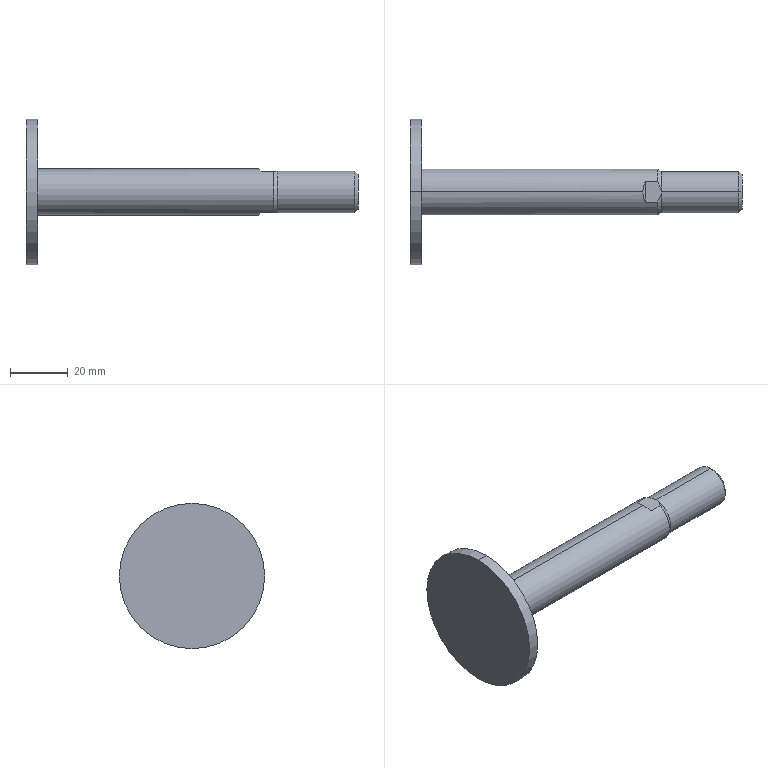Part | SolidWorks | features BaseBody 1 | 1 solid | 17 faces | box 115.2 x 50.4 x 50.4 mm | volume 29173 mm3 | plane 7 | cylinder 6 | cone 4 | commonest cylinder face diameters 14.4 x2 16 x2 50.4 x2
STEP:
#1=CARTESIAN_POINT('',(57.047,410.487,45.8));
#2=VERTEX_POINT('',#1);
#3=CARTESIAN_POINT('',(56.247,407.,45.));
#4=VERTEX_POINT('',#3);
#5=CARTESIAN_POINT('',(57.047,410.487,45.8));
#6=CARTESIAN_POINT('',(56.518,409.395,45.271));
#7=CARTESIAN_POINT('',(56.247,408.213,45.));
#8=CARTESIAN_POINT('',(56.247,407.,45.));
#9=(BOUNDED_CURVE()B_SPLINE_CURVE(3,(#5,#6,#7,#8),.UNSPECIFIED.,.F.,.F.)B_SPLINE_CURVE_WITH_KNOTS((4,4),(5.832,6.283),.UNSPECIFIED.)CURVE()GEOMETRIC_REPRESENTATION_ITEM()RATIONAL_B_SPLINE_CURVE((1.,0.9831,0.9831,1.))REPRESENTATION_ITEM(''));
#10=EDGE_CURVE('',#2,#4,#9,.T.);
#11=ORIENTED_EDGE('',*,*,#10,.T.);
#12=CARTESIAN_POINT('',(-20.553,407.,45.));
#13=VERTEX_POINT('',#12);
#14=CARTESIAN_POINT('',(-184.553,407.,45.));
#15=DIRECTION('',(-1.,0.,0.));
#16=VECTOR('',#15,1000.);
#17=LINE('',#14,#16);
#18=EDGE_CURVE('',#4,#13,#17,.T.);
#19=ORIENTED_EDGE('',*,*,#18,.T.);
#20=CARTESIAN_POINT('',(-20.553,407.,61.));
#21=VERTEX_POINT('',#20);
#22=CARTESIAN_POINT('',(-20.553,407.,53.));
#23=DIRECTION('',(1.,0.,0.));
#24=DIRECTION('',(0.,0.,1.));
#25=AXIS2_PLACEMENT_3D('',#22,#23,#24);
#26=CIRCLE('',#25,8.);
#27=EDGE_CURVE('',#13,#21,#26,.T.);
#28=ORIENTED_EDGE('',*,*,#27,.T.);
#29=CARTESIAN_POINT('',(56.247,407.,61.));
#30=VERTEX_POINT('',#29);
#31=CARTESIAN_POINT('',(-184.553,407.,61.));
#32=DIRECTION('',(-1.,0.,0.));
#33=VECTOR('',#32,1000.);
#34=LINE('',#31,#33);
#35=EDGE_CURVE('',#30,#21,#34,.T.);
#36=ORIENTED_EDGE('',*,*,#35,.F.);
#37=CARTESIAN_POINT('',(57.047,410.487,60.2));
#38=VERTEX_POINT('',#37);
#39=CARTESIAN_POINT('',(56.247,407.,61.));
#40=CARTESIAN_POINT('',(56.247,408.213,61.));
#41=CARTESIAN_POINT('',(56.518,409.395,60.729));
#42=CARTESIAN_POINT('',(57.047,410.487,60.2));
#43=(BOUNDED_CURVE()B_SPLINE_CURVE(3,(#39,#40,#41,#42),.UNSPECIFIED.,.F.,.F.)B_SPLINE_CURVE_WITH_KNOTS((4,4),(0.,0.451),.UNSPECIFIED.)CURVE()GEOMETRIC_REPRESENTATION_ITEM()RATIONAL_B_SPLINE_CURVE((1.,0.9831,0.9831,1.))REPRESENTATION_ITEM(''));
#44=EDGE_CURVE('',#30,#38,#43,.T.);
#45=ORIENTED_EDGE('',*,*,#44,.T.);
#46=CARTESIAN_POINT('',(61.261,410.487,60.2));
#47=VERTEX_POINT('',#46);
#48=CARTESIAN_POINT('',(-184.553,410.487,60.2));
#49=DIRECTION('',(1.,0.,0.));
#50=VECTOR('',#49,1000.);
#51=LINE('',#48,#50);
#52=EDGE_CURVE('',#38,#47,#51,.T.);
#53=ORIENTED_EDGE('',*,*,#52,.T.);
#54=CARTESIAN_POINT('',(61.261,410.487,45.8));
#55=VERTEX_POINT('',#54);
#56=CARTESIAN_POINT('',(61.261,407.,53.));
#57=DIRECTION('',(-1.,0.,0.));
#58=DIRECTION('',(0.,0.,1.));
#59=AXIS2_PLACEMENT_3D('',#56,#57,#58);
#60=CIRCLE('',#59,8.);
#61=EDGE_CURVE('',#47,#55,#60,.T.);
#62=ORIENTED_EDGE('',*,*,#61,.T.);
#63=CARTESIAN_POINT('',(-184.553,410.487,45.8));
#64=DIRECTION('',(-1.,0.,0.));
#65=VECTOR('',#64,1000.);
#66=LINE('',#63,#65);
#67=EDGE_CURVE('',#55,#2,#66,.T.);
#68=ORIENTED_EDGE('',*,*,#67,.T.);
#69=EDGE_LOOP('',(#11,#19,#28,#36,#45,#53,#62,#68));
#70=FACE_OUTER_BOUND('',#69,.T.);
#71=CARTESIAN_POINT('',(-184.553,407.,53.));
#72=DIRECTION('',(-1.,0.,0.));
#73=DIRECTION('',(0.,0.,1.));
#74=AXIS2_PLACEMENT_3D('',#71,#72,#73);
#75=CYLINDRICAL_SURFACE('',#74,8.);
#76=ADVANCED_FACE('',(#70),#75,.T.);
#77=CARTESIAN_POINT('',(-20.553,407.,78.2));
#78=VERTEX_POINT('',#77);
#79=CARTESIAN_POINT('',(-20.553,407.,27.8));
#80=VERTEX_POINT('',#79);
#81=CARTESIAN_POINT('',(-20.553,407.,53.));
#82=DIRECTION('',(-1.,0.,0.));
#83=DIRECTION('',(0.,0.,1.));
#84=AXIS2_PLACEMENT_3D('',#81,#82,#83);
#85=CIRCLE('',#84,25.2);
#86=EDGE_CURVE('',#78,#80,#85,.T.);
#87=ORIENTED_EDGE('',*,*,#86,.T.);
#88=CARTESIAN_POINT('',(-24.553,407.,27.8));
#89=VERTEX_POINT('',#88);
#90=CARTESIAN_POINT('',(-24.553,407.,27.8));
#91=DIRECTION('',(-1.,0.,0.));
#92=VECTOR('',#91,1000.);
#93=LINE('',#90,#92);
#94=EDGE_CURVE('',#80,#89,#93,.T.);
#95=ORIENTED_EDGE('',*,*,#94,.T.);
#96=CARTESIAN_POINT('',(-24.553,407.,78.2));
#97=VERTEX_POINT('',#96);
#98=CARTESIAN_POINT('',(-24.553,407.,53.));
#99=DIRECTION('',(1.,0.,0.));
#100=DIRECTION('',(0.,0.,1.));
#101=AXIS2_PLACEMENT_3D('',#98,#99,#100);
#102=CIRCLE('',#101,25.2);
#103=EDGE_CURVE('',#89,#97,#102,.T.);
#104=ORIENTED_EDGE('',*,*,#103,.T.);
#105=CARTESIAN_POINT('',(-24.553,407.,78.2));
#106=DIRECTION('',(-1.,0.,0.));
#107=VECTOR('',#106,1000.);
#108=LINE('',#105,#107);
#109=EDGE_CURVE('',#78,#97,#108,.T.);
#110=ORIENTED_EDGE('',*,*,#109,.F.);
#111=EDGE_LOOP('',(#87,#95,#104,#110));
#112=FACE_OUTER_BOUND('',#111,.T.);
#113=CARTESIAN_POINT('',(-24.553,407.,53.));
#114=DIRECTION('',(-1.,0.,0.));
#115=DIRECTION('',(0.,0.,1.));
#116=AXIS2_PLACEMENT_3D('',#113,#114,#115);
#117=CYLINDRICAL_SURFACE('',#116,25.2);
#118=ADVANCED_FACE('',(#112),#117,.T.);
#119=CARTESIAN_POINT('',(89.447,407.,60.2));
#120=VERTEX_POINT('',#119);
#121=CARTESIAN_POINT('',(89.447,407.,45.8));
#122=VERTEX_POINT('',#121);
#123=CARTESIAN_POINT('',(89.447,407.,53.));
#124=DIRECTION('',(-1.,0.,0.));
#125=DIRECTION('',(0.,0.,1.));
#126=AXIS2_PLACEMENT_3D('',#123,#124,#125);
#127=CIRCLE('',#126,7.2);
#128=EDGE_CURVE('',#120,#122,#127,.T.);
#129=ORIENTED_EDGE('',*,*,#128,.T.);
#130=CARTESIAN_POINT('',(62.647,407.,45.8));
#131=VERTEX_POINT('',#130);
#132=CARTESIAN_POINT('',(65.047,407.,45.8));
#133=DIRECTION('',(-1.,0.,0.));
#134=VECTOR('',#133,1000.);
#135=LINE('',#132,#134);
#136=EDGE_CURVE('',#122,#131,#135,.T.);
#137=ORIENTED_EDGE('',*,*,#136,.T.);
#138=CARTESIAN_POINT('',(62.647,407.,60.2));
#139=VERTEX_POINT('',#138);
#140=CARTESIAN_POINT('',(62.647,407.,53.));
#141=DIRECTION('',(-1.,0.,0.));
#142=DIRECTION('',(0.,0.,1.));
#143=AXIS2_PLACEMENT_3D('',#140,#141,#142);
#144=CIRCLE('',#143,7.2);
#145=EDGE_CURVE('',#139,#131,#144,.T.);
#146=ORIENTED_EDGE('',*,*,#145,.F.);
#147=CARTESIAN_POINT('',(65.047,407.,60.2));
#148=DIRECTION('',(-1.,0.,0.));
#149=VECTOR('',#148,1000.);
#150=LINE('',#147,#149);
#151=EDGE_CURVE('',#120,#139,#150,.T.);
#152=ORIENTED_EDGE('',*,*,#151,.F.);
#153=EDGE_LOOP('',(#129,#137,#146,#152));
#154=FACE_OUTER_BOUND('',#153,.T.);
#155=CARTESIAN_POINT('',(65.047,407.,53.));
#156=DIRECTION('',(-1.,0.,0.));
#157=DIRECTION('',(0.,0.,1.));
#158=AXIS2_PLACEMENT_3D('',#155,#156,#157);
#159=CYLINDRICAL_SURFACE('',#158,7.2);
#160=ADVANCED_FACE('',(#154),#159,.T.);
#161=CARTESIAN_POINT('',(90.647,407.,59.));
#162=VERTEX_POINT('',#161);
#163=CARTESIAN_POINT('',(90.647,407.,47.));
#164=VERTEX_POINT('',#163);
#165=CARTESIAN_POINT('',(90.647,407.,53.));
#166=DIRECTION('',(-1.,0.,0.));
#167=DIRECTION('',(0.,0.,1.));
#168=AXIS2_PLACEMENT_3D('',#165,#166,#167);
#169=CIRCLE('',#168,6.);
#170=EDGE_CURVE('',#162,#164,#169,.T.);
#171=ORIENTED_EDGE('',*,*,#170,.T.);
#172=CARTESIAN_POINT('',(89.447,407.,45.8));
#173=DIRECTION('',(-0.7071,0.,-0.7071));
#174=VECTOR('',#173,1000.);
#175=LINE('',#172,#174);
#176=EDGE_CURVE('',#164,#122,#175,.T.);
#177=ORIENTED_EDGE('',*,*,#176,.T.);
#178=ORIENTED_EDGE('',*,*,#128,.F.);
#179=CARTESIAN_POINT('',(89.447,407.,60.2));
#180=DIRECTION('',(-0.7071,0.,0.7071));
#181=VECTOR('',#180,1000.);
#182=LINE('',#179,#181);
#183=EDGE_CURVE('',#162,#120,#182,.T.);
#184=ORIENTED_EDGE('',*,*,#183,.F.);
#185=EDGE_LOOP('',(#171,#177,#178,#184));
#186=FACE_OUTER_BOUND('',#185,.T.);
#187=CARTESIAN_POINT('',(89.447,407.,53.));
#188=DIRECTION('',(-1.,0.,0.));
#189=DIRECTION('',(0.,0.,1.));
#190=AXIS2_PLACEMENT_3D('',#187,#188,#189);
#191=CONICAL_SURFACE('',#190,7.2,0.7854);
#192=ADVANCED_FACE('',(#186),#191,.T.);
#193=ORIENTED_EDGE('',*,*,#18,.F.);
#194=CARTESIAN_POINT('',(57.047,403.513,45.8));
#195=VERTEX_POINT('',#194);
#196=CARTESIAN_POINT('',(56.247,407.,45.));
#197=CARTESIAN_POINT('',(56.247,405.787,45.));
#198=CARTESIAN_POINT('',(56.518,404.605,45.271));
#199=CARTESIAN_POINT('',(57.047,403.513,45.8));
#200=(BOUNDED_CURVE()B_SPLINE_CURVE(3,(#196,#197,#198,#199),.UNSPECIFIED.,.F.,.F.)B_SPLINE_CURVE_WITH_KNOTS((4,4),(0.,0.451),.UNSPECIFIED.)CURVE()GEOMETRIC_REPRESENTATION_ITEM()RATIONAL_B_SPLINE_CURVE((1.,0.9831,0.9831,1.))REPRESENTATION_ITEM(''));
#201=EDGE_CURVE('',#4,#195,#200,.T.);
#202=ORIENTED_EDGE('',*,*,#201,.T.);
#203=CARTESIAN_POINT('',(61.261,403.513,45.8));
#204=VERTEX_POINT('',#203);
#205=CARTESIAN_POINT('',(-184.553,403.513,45.8));
#206=DIRECTION('',(1.,0.,0.));
#207=VECTOR('',#206,1000.);
#208=LINE('',#205,#207);
#209=EDGE_CURVE('',#195,#204,#208,.T.);
#210=ORIENTED_EDGE('',*,*,#209,.T.);
#211=CARTESIAN_POINT('',(61.261,403.513,60.2));
#212=VERTEX_POINT('',#211);
#213=CARTESIAN_POINT('',(61.261,407.,53.));
#214=DIRECTION('',(-1.,0.,0.));
#215=DIRECTION('',(0.,0.,1.));
#216=AXIS2_PLACEMENT_3D('',#213,#214,#215);
#217=CIRCLE('',#216,8.);
#218=EDGE_CURVE('',#204,#212,#217,.T.);
#219=ORIENTED_EDGE('',*,*,#218,.T.);
#220=CARTESIAN_POINT('',(57.047,403.513,60.2));
#221=VERTEX_POINT('',#220);
#222=CARTESIAN_POINT('',(-184.553,403.513,60.2));
#223=DIRECTION('',(-1.,0.,0.));
#224=VECTOR('',#223,1000.);
#225=LINE('',#222,#224);
#226=EDGE_CURVE('',#212,#221,#225,.T.);
#227=ORIENTED_EDGE('',*,*,#226,.T.);
#228=CARTESIAN_POINT('',(57.047,403.513,60.2));
#229=CARTESIAN_POINT('',(56.518,404.605,60.729));
#230=CARTESIAN_POINT('',(56.247,405.787,61.));
#231=CARTESIAN_POINT('',(56.247,407.,61.));
#232=(BOUNDED_CURVE()B_SPLINE_CURVE(3,(#228,#229,#230,#231),.UNSPECIFIED.,.F.,.T.)B_SPLINE_CURVE_WITH_KNOTS((4,4),(5.832,6.283),.UNSPECIFIED.)CURVE()GEOMETRIC_REPRESENTATION_ITEM()RATIONAL_B_SPLINE_CURVE((1.,0.9831,0.9831,1.))REPRESENTATION_ITEM(''));
#233=EDGE_CURVE('',#221,#30,#232,.T.);
#234=ORIENTED_EDGE('',*,*,#233,.T.);
#235=ORIENTED_EDGE('',*,*,#35,.T.);
#236=CARTESIAN_POINT('',(-20.553,407.,53.));
#237=DIRECTION('',(1.,0.,0.));
#238=DIRECTION('',(0.,0.,1.));
#239=AXIS2_PLACEMENT_3D('',#236,#237,#238);
#240=CIRCLE('',#239,8.);
#241=EDGE_CURVE('',#21,#13,#240,.T.);
#242=ORIENTED_EDGE('',*,*,#241,.T.);
#243=EDGE_LOOP('',(#193,#202,#210,#219,#227,#234,#235,#242));
#244=FACE_OUTER_BOUND('',#243,.T.);
#245=CARTESIAN_POINT('',(-184.553,407.,53.));
#246=DIRECTION('',(-1.,0.,0.));
#247=DIRECTION('',(0.,0.,1.));
#248=AXIS2_PLACEMENT_3D('',#245,#246,#247);
#249=CYLINDRICAL_SURFACE('',#248,8.);
#250=ADVANCED_FACE('',(#244),#249,.T.);
#251=ORIENTED_EDGE('',*,*,#241,.F.);
#252=ORIENTED_EDGE('',*,*,#27,.F.);
#253=EDGE_LOOP('',(#251,#252));
#254=FACE_BOUND('',#253,.T.);
#255=ORIENTED_EDGE('',*,*,#86,.F.);
#256=CARTESIAN_POINT('',(-20.553,407.,53.));
#257=DIRECTION('',(-1.,0.,0.));
#258=DIRECTION('',(0.,0.,1.));
#259=AXIS2_PLACEMENT_3D('',#256,#257,#258);
#260=CIRCLE('',#259,25.2);
#261=EDGE_CURVE('',#80,#78,#260,.T.);
#262=ORIENTED_EDGE('',*,*,#261,.F.);
#263=EDGE_LOOP('',(#255,#262));
#264=FACE_OUTER_BOUND('',#263,.T.);
#265=CARTESIAN_POINT('',(-20.553,399.,53.));
#266=DIRECTION('',(-1.,0.,0.));
#267=DIRECTION('',(0.,0.,1.));
#268=AXIS2_PLACEMENT_3D('',#265,#266,#267);
#269=PLANE('',#268);
#270=ADVANCED_FACE('',(#254,#264),#269,.F.);
#271=CARTESIAN_POINT('',(57.047,379.,60.2));
#272=DIRECTION('',(0.,1.,0.));
#273=VECTOR('',#272,1000.);
#274=LINE('',#271,#273);
#275=EDGE_CURVE('',#221,#38,#274,.T.);
#276=ORIENTED_EDGE('',*,*,#275,.T.);
#277=ORIENTED_EDGE('',*,*,#44,.F.);
#278=ORIENTED_EDGE('',*,*,#233,.F.);
#279=EDGE_LOOP('',(#276,#277,#278));
#280=FACE_OUTER_BOUND('',#279,.T.);
#281=CARTESIAN_POINT('',(53.047,379.,64.2));
#282=DIRECTION('',(0.7071,0.,0.7071));
#283=DIRECTION('',(0.7071,0.,-0.7071));
#284=AXIS2_PLACEMENT_3D('',#281,#282,#283);
#285=PLANE('',#284);
#286=ADVANCED_FACE('',(#280),#285,.T.);
#287=CARTESIAN_POINT('',(62.647,407.,60.2));
#288=CARTESIAN_POINT('',(62.647,407.322,60.2));
#289=CARTESIAN_POINT('',(62.609,407.637,60.2));
#290=CARTESIAN_POINT('',(62.47,408.255,60.2));
#291=CARTESIAN_POINT('',(62.367,408.56,60.2));
#292=CARTESIAN_POINT('',(61.987,409.44,60.2));
#293=CARTESIAN_POINT('',(61.646,409.977,60.2));
#294=CARTESIAN_POINT('',(61.261,410.487,60.2));
#295=B_SPLINE_CURVE_WITH_KNOTS('',3,(#287,#288,#289,#290,#291,#292,#293,#294),.UNSPECIFIED.,.F.,.F.,(4,2,2,4),(0.,0.000949,0.001898,0.003796),.UNSPECIFIED.);
#296=EDGE_CURVE('',#139,#47,#295,.T.);
#297=ORIENTED_EDGE('',*,*,#296,.T.);
#298=ORIENTED_EDGE('',*,*,#52,.F.);
#299=ORIENTED_EDGE('',*,*,#275,.F.);
#300=ORIENTED_EDGE('',*,*,#226,.F.);
#301=CARTESIAN_POINT('',(61.261,403.513,60.2));
#302=CARTESIAN_POINT('',(61.646,404.023,60.2));
#303=CARTESIAN_POINT('',(61.984,404.557,60.2));
#304=CARTESIAN_POINT('',(62.361,405.426,60.2));
#305=CARTESIAN_POINT('',(62.465,405.73,60.2));
#306=CARTESIAN_POINT('',(62.609,406.358,60.2));
#307=CARTESIAN_POINT('',(62.647,406.677,60.2));
#308=CARTESIAN_POINT('',(62.647,407.,60.2));
#309=B_SPLINE_CURVE_WITH_KNOTS('',3,(#301,#302,#303,#304,#305,#306,#307,#308),.UNSPECIFIED.,.F.,.F.,(4,2,2,4),(0.,0.00189,0.002835,0.00378),.UNSPECIFIED.);
#310=EDGE_CURVE('',#212,#139,#309,.T.);
#311=ORIENTED_EDGE('',*,*,#310,.T.);
#312=EDGE_LOOP('',(#297,#298,#299,#300,#311));
#313=FACE_OUTER_BOUND('',#312,.T.);
#314=CARTESIAN_POINT('',(57.047,379.,60.2));
#315=DIRECTION('',(0.,0.,1.));
#316=DIRECTION('',(1.,0.,0.));
#317=AXIS2_PLACEMENT_3D('',#314,#315,#316);
#318=PLANE('',#317);
#319=ADVANCED_FACE('',(#313),#318,.T.);
#320=CARTESIAN_POINT('',(61.261,403.513,45.8));
#321=CARTESIAN_POINT('',(61.646,404.023,45.8));
#322=CARTESIAN_POINT('',(61.984,404.557,45.8));
#323=CARTESIAN_POINT('',(62.361,405.426,45.8));
#324=CARTESIAN_POINT('',(62.465,405.73,45.8));
#325=CARTESIAN_POINT('',(62.609,406.358,45.8));
#326=CARTESIAN_POINT('',(62.647,406.677,45.8));
#327=CARTESIAN_POINT('',(62.647,407.,45.8));
#328=B_SPLINE_CURVE_WITH_KNOTS('',3,(#320,#321,#322,#323,#324,#325,#326,#327),.UNSPECIFIED.,.F.,.F.,(4,2,2,4),(0.,0.00189,0.002835,0.00378),.UNSPECIFIED.);
#329=EDGE_CURVE('',#204,#131,#328,.T.);
#330=ORIENTED_EDGE('',*,*,#329,.T.);
#331=CARTESIAN_POINT('',(62.647,407.,53.));
#332=DIRECTION('',(-1.,0.,0.));
#333=DIRECTION('',(0.,0.,1.));
#334=AXIS2_PLACEMENT_3D('',#331,#332,#333);
#335=CIRCLE('',#334,7.2);
#336=EDGE_CURVE('',#131,#139,#335,.T.);
#337=ORIENTED_EDGE('',*,*,#336,.T.);
#338=ORIENTED_EDGE('',*,*,#310,.F.);
#339=ORIENTED_EDGE('',*,*,#218,.F.);
#340=EDGE_LOOP('',(#330,#337,#338,#339));
#341=FACE_OUTER_BOUND('',#340,.T.);
#342=CARTESIAN_POINT('',(61.261,407.,53.));
#343=DIRECTION('',(-1.,0.,0.));
#344=DIRECTION('',(0.,0.,1.));
#345=AXIS2_PLACEMENT_3D('',#342,#343,#344);
#346=CONICAL_SURFACE('',#345,8.,0.5236);
#347=ADVANCED_FACE('',(#341),#346,.T.);
#348=ORIENTED_EDGE('',*,*,#329,.F.);
#349=ORIENTED_EDGE('',*,*,#209,.F.);
#350=CARTESIAN_POINT('',(57.047,379.,45.8));
#351=DIRECTION('',(0.,1.,0.));
#352=VECTOR('',#351,1000.);
#353=LINE('',#350,#352);
#354=EDGE_CURVE('',#195,#2,#353,.T.);
#355=ORIENTED_EDGE('',*,*,#354,.T.);
#356=ORIENTED_EDGE('',*,*,#67,.F.);
#357=CARTESIAN_POINT('',(61.261,410.487,45.8));
#358=CARTESIAN_POINT('',(61.646,409.977,45.8));
#359=CARTESIAN_POINT('',(61.984,409.443,45.8));
#360=CARTESIAN_POINT('',(62.361,408.574,45.8));
#361=CARTESIAN_POINT('',(62.465,408.27,45.8));
#362=CARTESIAN_POINT('',(62.609,407.642,45.8));
#363=CARTESIAN_POINT('',(62.647,407.323,45.8));
#364=CARTESIAN_POINT('',(62.647,407.,45.8));
#365=B_SPLINE_CURVE_WITH_KNOTS('',3,(#357,#358,#359,#360,#361,#362,#363,#364),.UNSPECIFIED.,.F.,.F.,(4,2,2,4),(0.,0.00189,0.002835,0.00378),.UNSPECIFIED.);
#366=EDGE_CURVE('',#55,#131,#365,.T.);
#367=ORIENTED_EDGE('',*,*,#366,.T.);
#368=EDGE_LOOP('',(#348,#349,#355,#356,#367));
#369=FACE_OUTER_BOUND('',#368,.T.);
#370=CARTESIAN_POINT('',(90.647,379.,45.8));
#371=DIRECTION('',(0.,0.,-1.));
#372=DIRECTION('',(-1.,0.,0.));
#373=AXIS2_PLACEMENT_3D('',#370,#371,#372);
#374=PLANE('',#373);
#375=ADVANCED_FACE('',(#369),#374,.T.);
#376=ORIENTED_EDGE('',*,*,#10,.F.);
#377=ORIENTED_EDGE('',*,*,#354,.F.);
#378=ORIENTED_EDGE('',*,*,#201,.F.);
#379=EDGE_LOOP('',(#376,#377,#378));
#380=FACE_OUTER_BOUND('',#379,.T.);
#381=CARTESIAN_POINT('',(57.047,379.,45.8));
#382=DIRECTION('',(0.7071,0.,-0.7071));
#383=DIRECTION('',(-0.7071,0.,-0.7071));
#384=AXIS2_PLACEMENT_3D('',#381,#382,#383);
#385=PLANE('',#384);
#386=ADVANCED_FACE('',(#380),#385,.T.);
#387=ORIENTED_EDGE('',*,*,#94,.F.);
#388=ORIENTED_EDGE('',*,*,#261,.T.);
#389=ORIENTED_EDGE('',*,*,#109,.T.);
#390=CARTESIAN_POINT('',(-24.553,407.,53.));
#391=DIRECTION('',(1.,0.,0.));
#392=DIRECTION('',(0.,0.,1.));
#393=AXIS2_PLACEMENT_3D('',#390,#391,#392);
#394=CIRCLE('',#393,25.2);
#395=EDGE_CURVE('',#97,#89,#394,.T.);
#396=ORIENTED_EDGE('',*,*,#395,.T.);
#397=EDGE_LOOP('',(#387,#388,#389,#396));
#398=FACE_OUTER_BOUND('',#397,.T.);
#399=CARTESIAN_POINT('',(-24.553,407.,53.));
#400=DIRECTION('',(-1.,0.,0.));
#401=DIRECTION('',(0.,0.,1.));
#402=AXIS2_PLACEMENT_3D('',#399,#400,#401);
#403=CYLINDRICAL_SURFACE('',#402,25.2);
#404=ADVANCED_FACE('',(#398),#403,.T.);
#405=ORIENTED_EDGE('',*,*,#366,.F.);
#406=ORIENTED_EDGE('',*,*,#61,.F.);
#407=ORIENTED_EDGE('',*,*,#296,.F.);
#408=ORIENTED_EDGE('',*,*,#145,.T.);
#409=EDGE_LOOP('',(#405,#406,#407,#408));
#410=FACE_OUTER_BOUND('',#409,.T.);
#411=CARTESIAN_POINT('',(61.261,407.,53.));
#412=DIRECTION('',(-1.,0.,0.));
#413=DIRECTION('',(0.,-1.,0.));
#414=AXIS2_PLACEMENT_3D('',#411,#412,#413);
#415=CONICAL_SURFACE('',#414,8.,0.5236);
#416=ADVANCED_FACE('',(#410),#415,.T.);
#417=ORIENTED_EDGE('',*,*,#136,.F.);
#418=CARTESIAN_POINT('',(89.447,407.,53.));
#419=DIRECTION('',(-1.,0.,0.));
#420=DIRECTION('',(0.,0.,1.));
#421=AXIS2_PLACEMENT_3D('',#418,#419,#420);
#422=CIRCLE('',#421,7.2);
#423=EDGE_CURVE('',#122,#120,#422,.T.);
#424=ORIENTED_EDGE('',*,*,#423,.T.);
#425=ORIENTED_EDGE('',*,*,#151,.T.);
#426=ORIENTED_EDGE('',*,*,#336,.F.);
#427=EDGE_LOOP('',(#417,#424,#425,#426));
#428=FACE_OUTER_BOUND('',#427,.T.);
#429=CARTESIAN_POINT('',(65.047,407.,53.));
#430=DIRECTION('',(-1.,0.,0.));
#431=DIRECTION('',(0.,0.,1.));
#432=AXIS2_PLACEMENT_3D('',#429,#430,#431);
#433=CYLINDRICAL_SURFACE('',#432,7.2);
#434=ADVANCED_FACE('',(#428),#433,.T.);
#435=ORIENTED_EDGE('',*,*,#395,.F.);
#436=ORIENTED_EDGE('',*,*,#103,.F.);
#437=EDGE_LOOP('',(#435,#436));
#438=FACE_OUTER_BOUND('',#437,.T.);
#439=CARTESIAN_POINT('',(-24.553,381.8,53.));
#440=DIRECTION('',(1.,0.,0.));
#441=DIRECTION('',(0.,0.,-1.));
#442=AXIS2_PLACEMENT_3D('',#439,#440,#441);
#443=PLANE('',#442);
#444=ADVANCED_FACE('',(#438),#443,.F.);
#445=ORIENTED_EDGE('',*,*,#176,.F.);
#446=CARTESIAN_POINT('',(90.647,407.,53.));
#447=DIRECTION('',(-1.,0.,0.));
#448=DIRECTION('',(0.,0.,1.));
#449=AXIS2_PLACEMENT_3D('',#446,#447,#448);
#450=CIRCLE('',#449,6.);
#451=EDGE_CURVE('',#164,#162,#450,.T.);
#452=ORIENTED_EDGE('',*,*,#451,.T.);
#453=ORIENTED_EDGE('',*,*,#183,.T.);
#454=ORIENTED_EDGE('',*,*,#423,.F.);
#455=EDGE_LOOP('',(#445,#452,#453,#454));
#456=FACE_OUTER_BOUND('',#455,.T.);
#457=CARTESIAN_POINT('',(89.447,407.,53.));
#458=DIRECTION('',(-1.,0.,0.));
#459=DIRECTION('',(0.,0.,1.));
#460=AXIS2_PLACEMENT_3D('',#457,#458,#459);
#461=CONICAL_SURFACE('',#460,7.2,0.7854);
#462=ADVANCED_FACE('',(#456),#461,.T.);
#463=ORIENTED_EDGE('',*,*,#170,.F.);
#464=ORIENTED_EDGE('',*,*,#451,.F.);
#465=EDGE_LOOP('',(#463,#464));
#466=FACE_OUTER_BOUND('',#465,.T.);
#467=CARTESIAN_POINT('',(90.647,407.,53.));
#468=DIRECTION('',(-1.,0.,0.));
#469=DIRECTION('',(0.,0.,1.));
#470=AXIS2_PLACEMENT_3D('',#467,#468,#469);
#471=PLANE('',#470);
#472=ADVANCED_FACE('',(#466),#471,.F.);
#473=CLOSED_SHELL('',(#76,#118,#160,#192,#250,#270,#286,#319,#347,#375,#386,#404,#416,#434,#444,#462,#472));
#474=MANIFOLD_SOLID_BREP('',#473);
#475=CARTESIAN_POINT('',(0.,0.,0.));
#476=DIRECTION('',(0.,0.,1.));
#477=DIRECTION('',(1.,0.,0.));
#478=AXIS2_PLACEMENT_3D('',#475,#476,#477);
#479=(LENGTH_UNIT()NAMED_UNIT(*)SI_UNIT(.MILLI.,.METRE.));
#480=UNCERTAINTY_MEASURE_WITH_UNIT(LENGTH_MEASURE(0.00001),#479,'','');
#481=(NAMED_UNIT(*)PLANE_ANGLE_UNIT()SI_UNIT($,.RADIAN.));
#482=(NAMED_UNIT(*)SI_UNIT($,.STERADIAN.)SOLID_ANGLE_UNIT());
#483=(GEOMETRIC_REPRESENTATION_CONTEXT(3)GLOBAL_UNCERTAINTY_ASSIGNED_CONTEXT((#480))GLOBAL_UNIT_ASSIGNED_CONTEXT((#479,#481,#482))REPRESENTATION_CONTEXT('',''));
#484=ADVANCED_BREP_SHAPE_REPRESENTATION('',(#474,#478),#483);